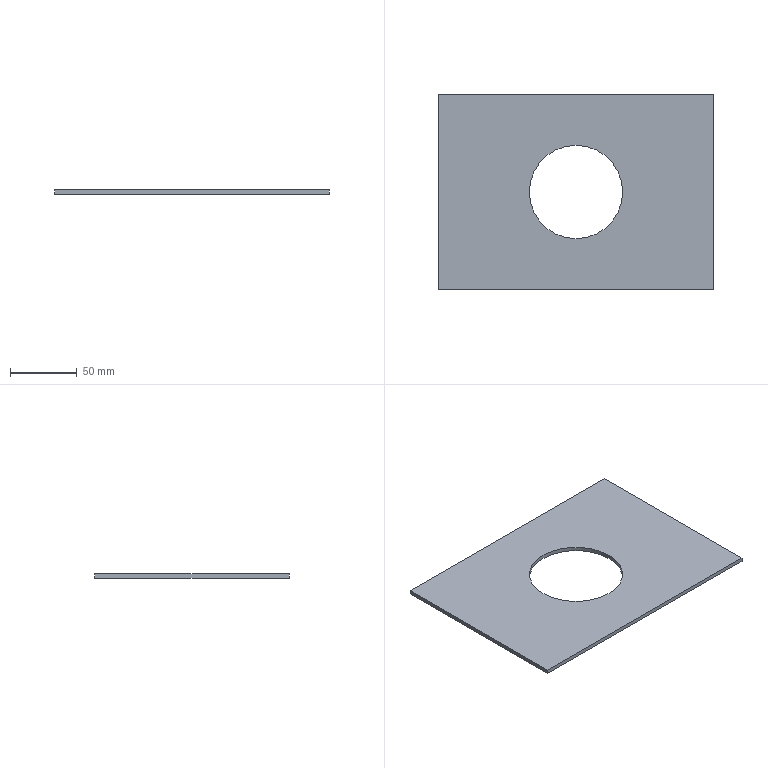Part | SolidWorks | features Extrusion 1, ICE 1 | 1 solid | 8 faces | box 206 x 146 x 3 mm | volume 78683 mm3 | plane 6 | cylinder 2 | commonest cylinder face diameters 70 x2
STEP:
#1=CARTESIAN_POINT('',(-35.,0.,-1.5));
#2=VERTEX_POINT('',#1);
#3=CARTESIAN_POINT('',(35.,0.,-1.5));
#4=VERTEX_POINT('',#3);
#5=CARTESIAN_POINT('',(0.,0.,-1.5));
#6=DIRECTION('',(0.,0.,1.));
#7=DIRECTION('',(1.,0.,0.));
#8=AXIS2_PLACEMENT_3D('',#5,#6,#7);
#9=CIRCLE('',#8,35.);
#10=EDGE_CURVE('',#2,#4,#9,.T.);
#11=ORIENTED_EDGE('',*,*,#10,.F.);
#12=CARTESIAN_POINT('',(-35.,0.,1.5));
#13=VERTEX_POINT('',#12);
#14=CARTESIAN_POINT('',(-35.,0.,-11.5));
#15=DIRECTION('',(0.,0.,1.));
#16=VECTOR('',#15,1000.);
#17=LINE('',#14,#16);
#18=EDGE_CURVE('',#2,#13,#17,.T.);
#19=ORIENTED_EDGE('',*,*,#18,.T.);
#20=CARTESIAN_POINT('',(35.,0.,1.5));
#21=VERTEX_POINT('',#20);
#22=CARTESIAN_POINT('',(0.,0.,1.5));
#23=DIRECTION('',(0.,0.,1.));
#24=DIRECTION('',(1.,0.,0.));
#25=AXIS2_PLACEMENT_3D('',#22,#23,#24);
#26=CIRCLE('',#25,35.);
#27=EDGE_CURVE('',#13,#21,#26,.T.);
#28=ORIENTED_EDGE('',*,*,#27,.T.);
#29=CARTESIAN_POINT('',(35.,0.,-11.5));
#30=DIRECTION('',(0.,0.,1.));
#31=VECTOR('',#30,1000.);
#32=LINE('',#29,#31);
#33=EDGE_CURVE('',#4,#21,#32,.T.);
#34=ORIENTED_EDGE('',*,*,#33,.F.);
#35=EDGE_LOOP('',(#11,#19,#28,#34));
#36=FACE_OUTER_BOUND('',#35,.T.);
#37=CARTESIAN_POINT('',(0.,0.,-11.5));
#38=DIRECTION('',(0.,0.,1.));
#39=DIRECTION('',(1.,0.,0.));
#40=AXIS2_PLACEMENT_3D('',#37,#38,#39);
#41=CYLINDRICAL_SURFACE('',#40,35.);
#42=ADVANCED_FACE('',(#36),#41,.F.);
#43=CARTESIAN_POINT('',(-103.,73.,1.5));
#44=VERTEX_POINT('',#43);
#45=CARTESIAN_POINT('',(-103.,-73.,1.5));
#46=VERTEX_POINT('',#45);
#47=CARTESIAN_POINT('',(-103.,73.,1.5));
#48=DIRECTION('',(0.,-1.,0.));
#49=VECTOR('',#48,1000.);
#50=LINE('',#47,#49);
#51=EDGE_CURVE('',#44,#46,#50,.T.);
#52=ORIENTED_EDGE('',*,*,#51,.F.);
#53=CARTESIAN_POINT('',(-103.,73.,-1.5));
#54=VERTEX_POINT('',#53);
#55=CARTESIAN_POINT('',(-103.,73.,-1.5));
#56=DIRECTION('',(0.,0.,1.));
#57=VECTOR('',#56,1000.);
#58=LINE('',#55,#57);
#59=EDGE_CURVE('',#54,#44,#58,.T.);
#60=ORIENTED_EDGE('',*,*,#59,.F.);
#61=CARTESIAN_POINT('',(-103.,-73.,-1.5));
#62=VERTEX_POINT('',#61);
#63=CARTESIAN_POINT('',(-103.,73.,-1.5));
#64=DIRECTION('',(0.,-1.,0.));
#65=VECTOR('',#64,1000.);
#66=LINE('',#63,#65);
#67=EDGE_CURVE('',#54,#62,#66,.T.);
#68=ORIENTED_EDGE('',*,*,#67,.T.);
#69=CARTESIAN_POINT('',(-103.,-73.,-1.5));
#70=DIRECTION('',(0.,0.,1.));
#71=VECTOR('',#70,1000.);
#72=LINE('',#69,#71);
#73=EDGE_CURVE('',#62,#46,#72,.T.);
#74=ORIENTED_EDGE('',*,*,#73,.T.);
#75=EDGE_LOOP('',(#52,#60,#68,#74));
#76=FACE_OUTER_BOUND('',#75,.T.);
#77=CARTESIAN_POINT('',(-103.,73.,-1.5));
#78=DIRECTION('',(-1.,0.,0.));
#79=DIRECTION('',(0.,0.,1.));
#80=AXIS2_PLACEMENT_3D('',#77,#78,#79);
#81=PLANE('',#80);
#82=ADVANCED_FACE('',(#76),#81,.T.);
#83=CARTESIAN_POINT('',(103.,73.,1.5));
#84=VERTEX_POINT('',#83);
#85=CARTESIAN_POINT('',(103.,73.,1.5));
#86=DIRECTION('',(-1.,0.,0.));
#87=VECTOR('',#86,1000.);
#88=LINE('',#85,#87);
#89=EDGE_CURVE('',#84,#44,#88,.T.);
#90=ORIENTED_EDGE('',*,*,#89,.F.);
#91=CARTESIAN_POINT('',(103.,73.,-1.5));
#92=VERTEX_POINT('',#91);
#93=CARTESIAN_POINT('',(103.,73.,-1.5));
#94=DIRECTION('',(0.,0.,1.));
#95=VECTOR('',#94,1000.);
#96=LINE('',#93,#95);
#97=EDGE_CURVE('',#92,#84,#96,.T.);
#98=ORIENTED_EDGE('',*,*,#97,.F.);
#99=CARTESIAN_POINT('',(103.,73.,-1.5));
#100=DIRECTION('',(-1.,0.,0.));
#101=VECTOR('',#100,1000.);
#102=LINE('',#99,#101);
#103=EDGE_CURVE('',#92,#54,#102,.T.);
#104=ORIENTED_EDGE('',*,*,#103,.T.);
#105=ORIENTED_EDGE('',*,*,#59,.T.);
#106=EDGE_LOOP('',(#90,#98,#104,#105));
#107=FACE_OUTER_BOUND('',#106,.T.);
#108=CARTESIAN_POINT('',(103.,73.,-1.5));
#109=DIRECTION('',(0.,1.,0.));
#110=DIRECTION('',(0.,0.,1.));
#111=AXIS2_PLACEMENT_3D('',#108,#109,#110);
#112=PLANE('',#111);
#113=ADVANCED_FACE('',(#107),#112,.T.);
#114=CARTESIAN_POINT('',(103.,-73.,1.5));
#115=VERTEX_POINT('',#114);
#116=CARTESIAN_POINT('',(103.,-73.,1.5));
#117=DIRECTION('',(0.,1.,0.));
#118=VECTOR('',#117,1000.);
#119=LINE('',#116,#118);
#120=EDGE_CURVE('',#115,#84,#119,.T.);
#121=ORIENTED_EDGE('',*,*,#120,.F.);
#122=CARTESIAN_POINT('',(103.,-73.,-1.5));
#123=VERTEX_POINT('',#122);
#124=CARTESIAN_POINT('',(103.,-73.,-1.5));
#125=DIRECTION('',(0.,0.,1.));
#126=VECTOR('',#125,1000.);
#127=LINE('',#124,#126);
#128=EDGE_CURVE('',#123,#115,#127,.T.);
#129=ORIENTED_EDGE('',*,*,#128,.F.);
#130=CARTESIAN_POINT('',(103.,-73.,-1.5));
#131=DIRECTION('',(0.,1.,0.));
#132=VECTOR('',#131,1000.);
#133=LINE('',#130,#132);
#134=EDGE_CURVE('',#123,#92,#133,.T.);
#135=ORIENTED_EDGE('',*,*,#134,.T.);
#136=ORIENTED_EDGE('',*,*,#97,.T.);
#137=EDGE_LOOP('',(#121,#129,#135,#136));
#138=FACE_OUTER_BOUND('',#137,.T.);
#139=CARTESIAN_POINT('',(103.,-73.,-1.5));
#140=DIRECTION('',(1.,0.,0.));
#141=DIRECTION('',(0.,0.,-1.));
#142=AXIS2_PLACEMENT_3D('',#139,#140,#141);
#143=PLANE('',#142);
#144=ADVANCED_FACE('',(#138),#143,.T.);
#145=CARTESIAN_POINT('',(-103.,-73.,1.5));
#146=DIRECTION('',(1.,0.,0.));
#147=VECTOR('',#146,1000.);
#148=LINE('',#145,#147);
#149=EDGE_CURVE('',#46,#115,#148,.T.);
#150=ORIENTED_EDGE('',*,*,#149,.F.);
#151=ORIENTED_EDGE('',*,*,#73,.F.);
#152=CARTESIAN_POINT('',(-103.,-73.,-1.5));
#153=DIRECTION('',(1.,0.,0.));
#154=VECTOR('',#153,1000.);
#155=LINE('',#152,#154);
#156=EDGE_CURVE('',#62,#123,#155,.T.);
#157=ORIENTED_EDGE('',*,*,#156,.T.);
#158=ORIENTED_EDGE('',*,*,#128,.T.);
#159=EDGE_LOOP('',(#150,#151,#157,#158));
#160=FACE_OUTER_BOUND('',#159,.T.);
#161=CARTESIAN_POINT('',(-103.,-73.,-1.5));
#162=DIRECTION('',(0.,-1.,0.));
#163=DIRECTION('',(0.,0.,-1.));
#164=AXIS2_PLACEMENT_3D('',#161,#162,#163);
#165=PLANE('',#164);
#166=ADVANCED_FACE('',(#160),#165,.T.);
#167=CARTESIAN_POINT('',(0.,0.,-1.5));
#168=DIRECTION('',(0.,0.,1.));
#169=DIRECTION('',(1.,0.,0.));
#170=AXIS2_PLACEMENT_3D('',#167,#168,#169);
#171=CIRCLE('',#170,35.);
#172=EDGE_CURVE('',#4,#2,#171,.T.);
#173=ORIENTED_EDGE('',*,*,#172,.T.);
#174=ORIENTED_EDGE('',*,*,#10,.T.);
#175=EDGE_LOOP('',(#173,#174));
#176=FACE_BOUND('',#175,.T.);
#177=ORIENTED_EDGE('',*,*,#67,.F.);
#178=ORIENTED_EDGE('',*,*,#103,.F.);
#179=ORIENTED_EDGE('',*,*,#134,.F.);
#180=ORIENTED_EDGE('',*,*,#156,.F.);
#181=EDGE_LOOP('',(#177,#178,#179,#180));
#182=FACE_OUTER_BOUND('',#181,.T.);
#183=CARTESIAN_POINT('',(0.,0.,-1.5));
#184=DIRECTION('',(0.,0.,1.));
#185=DIRECTION('',(1.,0.,0.));
#186=AXIS2_PLACEMENT_3D('',#183,#184,#185);
#187=PLANE('',#186);
#188=ADVANCED_FACE('',(#176,#182),#187,.F.);
#189=CARTESIAN_POINT('',(0.,0.,1.5));
#190=DIRECTION('',(0.,0.,1.));
#191=DIRECTION('',(1.,0.,0.));
#192=AXIS2_PLACEMENT_3D('',#189,#190,#191);
#193=CIRCLE('',#192,35.);
#194=EDGE_CURVE('',#21,#13,#193,.T.);
#195=ORIENTED_EDGE('',*,*,#194,.F.);
#196=ORIENTED_EDGE('',*,*,#27,.F.);
#197=EDGE_LOOP('',(#195,#196));
#198=FACE_BOUND('',#197,.T.);
#199=ORIENTED_EDGE('',*,*,#51,.T.);
#200=ORIENTED_EDGE('',*,*,#149,.T.);
#201=ORIENTED_EDGE('',*,*,#120,.T.);
#202=ORIENTED_EDGE('',*,*,#89,.T.);
#203=EDGE_LOOP('',(#199,#200,#201,#202));
#204=FACE_OUTER_BOUND('',#203,.T.);
#205=CARTESIAN_POINT('',(0.,0.,1.5));
#206=DIRECTION('',(0.,0.,1.));
#207=DIRECTION('',(1.,0.,0.));
#208=AXIS2_PLACEMENT_3D('',#205,#206,#207);
#209=PLANE('',#208);
#210=ADVANCED_FACE('',(#198,#204),#209,.T.);
#211=ORIENTED_EDGE('',*,*,#18,.F.);
#212=ORIENTED_EDGE('',*,*,#172,.F.);
#213=ORIENTED_EDGE('',*,*,#33,.T.);
#214=ORIENTED_EDGE('',*,*,#194,.T.);
#215=EDGE_LOOP('',(#211,#212,#213,#214));
#216=FACE_OUTER_BOUND('',#215,.T.);
#217=CARTESIAN_POINT('',(0.,0.,-11.5));
#218=DIRECTION('',(0.,0.,1.));
#219=DIRECTION('',(1.,0.,0.));
#220=AXIS2_PLACEMENT_3D('',#217,#218,#219);
#221=CYLINDRICAL_SURFACE('',#220,35.);
#222=ADVANCED_FACE('',(#216),#221,.F.);
#223=CLOSED_SHELL('',(#42,#82,#113,#144,#166,#188,#210,#222));
#224=MANIFOLD_SOLID_BREP('',#223);
#225=CARTESIAN_POINT('',(0.,0.,0.));
#226=DIRECTION('',(0.,0.,1.));
#227=DIRECTION('',(1.,0.,0.));
#228=AXIS2_PLACEMENT_3D('',#225,#226,#227);
#229=(LENGTH_UNIT()NAMED_UNIT(*)SI_UNIT(.MILLI.,.METRE.));
#230=UNCERTAINTY_MEASURE_WITH_UNIT(LENGTH_MEASURE(0.00001),#229,'','');
#231=(NAMED_UNIT(*)PLANE_ANGLE_UNIT()SI_UNIT($,.RADIAN.));
#232=(NAMED_UNIT(*)SI_UNIT($,.STERADIAN.)SOLID_ANGLE_UNIT());
#233=(GEOMETRIC_REPRESENTATION_CONTEXT(3)GLOBAL_UNCERTAINTY_ASSIGNED_CONTEXT((#230))GLOBAL_UNIT_ASSIGNED_CONTEXT((#229,#231,#232))REPRESENTATION_CONTEXT('',''));
#234=ADVANCED_BREP_SHAPE_REPRESENTATION('',(#224,#228),#233);